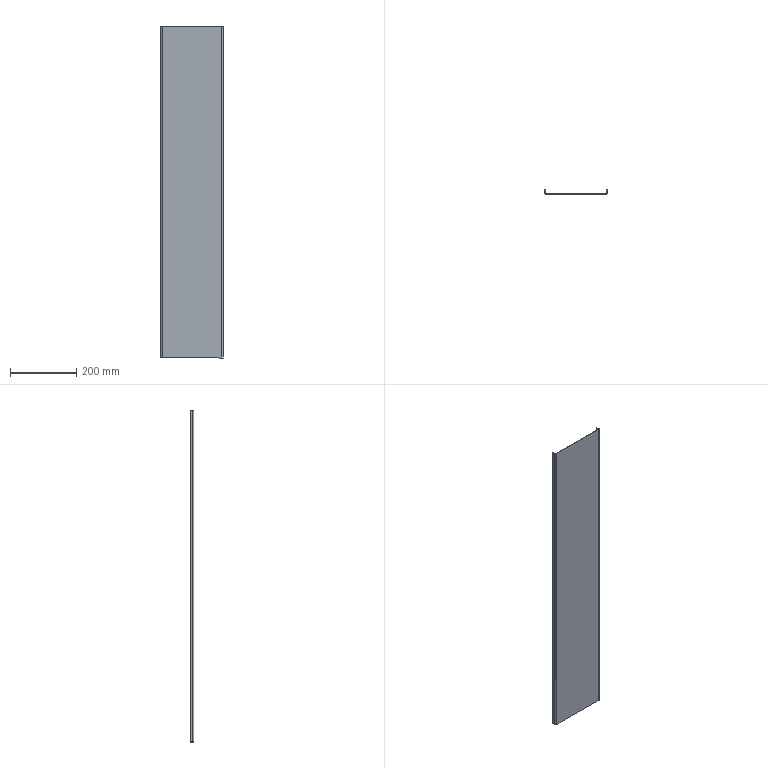Part | STEP file | HXGR200008-05-16 | 1 solid | 22 faces | box 187 x 12 x 1000 mm | volume 408850 mm3 | plane 18 | cylinder 4 | commonest cylinder face diameters 4 x2 8 x2
STEP:
#1=CARTESIAN_POINT('',(-91.5,2.,-1000.));
#2=VERTEX_POINT('',#1);
#3=CARTESIAN_POINT('',(-93.5,2.,-1000.));
#4=VERTEX_POINT('',#3);
#5=CARTESIAN_POINT('',(-91.5,2.,-1000.));
#6=DIRECTION('',(-1.,0.,0.));
#7=VECTOR('',#6,1000.);
#8=LINE('',#5,#7);
#9=EDGE_CURVE('',#2,#4,#8,.T.);
#10=ORIENTED_EDGE('',*,*,#9,.F.);
#11=CARTESIAN_POINT('',(-89.5,0.,-1000.));
#12=VERTEX_POINT('',#11);
#13=CARTESIAN_POINT('',(-89.5,2.,-1000.));
#14=DIRECTION('',(0.,0.,1.));
#15=DIRECTION('',(-1.,0.,0.));
#16=AXIS2_PLACEMENT_3D('',#13,#14,#15);
#17=CIRCLE('',#16,2.);
#18=EDGE_CURVE('',#2,#12,#17,.T.);
#19=ORIENTED_EDGE('',*,*,#18,.T.);
#20=CARTESIAN_POINT('',(-89.5,-2.,-1000.));
#21=VERTEX_POINT('',#20);
#22=CARTESIAN_POINT('',(-89.5,-2.,-1000.));
#23=DIRECTION('',(0.,1.,0.));
#24=VECTOR('',#23,1000.);
#25=LINE('',#22,#24);
#26=EDGE_CURVE('',#21,#12,#25,.T.);
#27=ORIENTED_EDGE('',*,*,#26,.F.);
#28=CARTESIAN_POINT('',(-89.5,2.,-1000.));
#29=DIRECTION('',(0.,0.,1.));
#30=DIRECTION('',(1.,0.,0.));
#31=AXIS2_PLACEMENT_3D('',#28,#29,#30);
#32=CIRCLE('',#31,4.);
#33=EDGE_CURVE('',#4,#21,#32,.T.);
#34=ORIENTED_EDGE('',*,*,#33,.F.);
#35=EDGE_LOOP('',(#10,#19,#27,#34));
#36=FACE_OUTER_BOUND('',#35,.T.);
#37=CARTESIAN_POINT('',(-91.5,2.,-1000.));
#38=DIRECTION('',(0.,0.,-1.));
#39=DIRECTION('',(-1.,0.,0.));
#40=AXIS2_PLACEMENT_3D('',#37,#38,#39);
#41=PLANE('',#40);
#42=ADVANCED_FACE('',(#36),#41,.T.);
#43=CARTESIAN_POINT('',(-91.5,10.,-1000.));
#44=VERTEX_POINT('',#43);
#45=CARTESIAN_POINT('',(-91.5,0.,-1000.));
#46=DIRECTION('',(0.,-1.,0.));
#47=VECTOR('',#46,1000.);
#48=LINE('',#45,#47);
#49=EDGE_CURVE('',#44,#2,#48,.T.);
#50=ORIENTED_EDGE('',*,*,#49,.T.);
#51=ORIENTED_EDGE('',*,*,#9,.T.);
#52=CARTESIAN_POINT('',(-93.5,10.,-1000.));
#53=VERTEX_POINT('',#52);
#54=CARTESIAN_POINT('',(-93.5,0.,-1000.));
#55=DIRECTION('',(0.,-1.,0.));
#56=VECTOR('',#55,1000.);
#57=LINE('',#54,#56);
#58=EDGE_CURVE('',#53,#4,#57,.T.);
#59=ORIENTED_EDGE('',*,*,#58,.F.);
#60=CARTESIAN_POINT('',(-93.5,10.,-1000.));
#61=DIRECTION('',(1.,0.,0.));
#62=VECTOR('',#61,1000.);
#63=LINE('',#60,#62);
#64=EDGE_CURVE('',#53,#44,#63,.T.);
#65=ORIENTED_EDGE('',*,*,#64,.T.);
#66=EDGE_LOOP('',(#50,#51,#59,#65));
#67=FACE_OUTER_BOUND('',#66,.T.);
#68=CARTESIAN_POINT('',(-89.5,-2.,-1000.));
#69=DIRECTION('',(0.,0.,-1.));
#70=DIRECTION('',(-1.,0.,0.));
#71=AXIS2_PLACEMENT_3D('',#68,#69,#70);
#72=PLANE('',#71);
#73=ADVANCED_FACE('',(#67),#72,.T.);
#74=CARTESIAN_POINT('',(-89.5,0.,0.));
#75=VERTEX_POINT('',#74);
#76=CARTESIAN_POINT('',(-89.5,-2.,0.));
#77=VERTEX_POINT('',#76);
#78=CARTESIAN_POINT('',(-89.5,0.,0.));
#79=DIRECTION('',(0.,-1.,0.));
#80=VECTOR('',#79,1000.);
#81=LINE('',#78,#80);
#82=EDGE_CURVE('',#75,#77,#81,.T.);
#83=ORIENTED_EDGE('',*,*,#82,.F.);
#84=CARTESIAN_POINT('',(-91.5,2.,0.));
#85=VERTEX_POINT('',#84);
#86=CARTESIAN_POINT('',(-89.5,2.,0.));
#87=DIRECTION('',(0.,0.,1.));
#88=DIRECTION('',(-1.,0.,0.));
#89=AXIS2_PLACEMENT_3D('',#86,#87,#88);
#90=CIRCLE('',#89,2.);
#91=EDGE_CURVE('',#85,#75,#90,.T.);
#92=ORIENTED_EDGE('',*,*,#91,.F.);
#93=CARTESIAN_POINT('',(-93.5,2.,0.));
#94=VERTEX_POINT('',#93);
#95=CARTESIAN_POINT('',(-93.5,2.,0.));
#96=DIRECTION('',(1.,0.,0.));
#97=VECTOR('',#96,1000.);
#98=LINE('',#95,#97);
#99=EDGE_CURVE('',#94,#85,#98,.T.);
#100=ORIENTED_EDGE('',*,*,#99,.F.);
#101=CARTESIAN_POINT('',(-89.5,2.,0.));
#102=DIRECTION('',(0.,0.,1.));
#103=DIRECTION('',(1.,0.,0.));
#104=AXIS2_PLACEMENT_3D('',#101,#102,#103);
#105=CIRCLE('',#104,4.);
#106=EDGE_CURVE('',#94,#77,#105,.T.);
#107=ORIENTED_EDGE('',*,*,#106,.T.);
#108=EDGE_LOOP('',(#83,#92,#100,#107));
#109=FACE_OUTER_BOUND('',#108,.T.);
#110=CARTESIAN_POINT('',(-89.5,0.,0.));
#111=DIRECTION('',(0.,0.,1.));
#112=DIRECTION('',(1.,0.,0.));
#113=AXIS2_PLACEMENT_3D('',#110,#111,#112);
#114=PLANE('',#113);
#115=ADVANCED_FACE('',(#109),#114,.T.);
#116=CARTESIAN_POINT('',(89.5,0.,0.));
#117=VERTEX_POINT('',#116);
#118=CARTESIAN_POINT('',(-91.5,0.,0.));
#119=DIRECTION('',(1.,0.,0.));
#120=VECTOR('',#119,1000.);
#121=LINE('',#118,#120);
#122=EDGE_CURVE('',#75,#117,#121,.T.);
#123=ORIENTED_EDGE('',*,*,#122,.F.);
#124=ORIENTED_EDGE('',*,*,#82,.T.);
#125=CARTESIAN_POINT('',(89.5,-2.,0.));
#126=VERTEX_POINT('',#125);
#127=CARTESIAN_POINT('',(-91.5,-2.,0.));
#128=DIRECTION('',(1.,0.,0.));
#129=VECTOR('',#128,1000.);
#130=LINE('',#127,#129);
#131=EDGE_CURVE('',#77,#126,#130,.T.);
#132=ORIENTED_EDGE('',*,*,#131,.T.);
#133=CARTESIAN_POINT('',(89.5,-2.,0.));
#134=DIRECTION('',(0.,1.,0.));
#135=VECTOR('',#134,1000.);
#136=LINE('',#133,#135);
#137=EDGE_CURVE('',#126,#117,#136,.T.);
#138=ORIENTED_EDGE('',*,*,#137,.T.);
#139=EDGE_LOOP('',(#123,#124,#132,#138));
#140=FACE_OUTER_BOUND('',#139,.T.);
#141=CARTESIAN_POINT('',(-93.5,2.,0.));
#142=DIRECTION('',(0.,0.,1.));
#143=DIRECTION('',(1.,0.,0.));
#144=AXIS2_PLACEMENT_3D('',#141,#142,#143);
#145=PLANE('',#144);
#146=ADVANCED_FACE('',(#140),#145,.T.);
#147=CARTESIAN_POINT('',(89.5,0.,-1000.));
#148=VERTEX_POINT('',#147);
#149=CARTESIAN_POINT('',(89.5,-2.,-1000.));
#150=VERTEX_POINT('',#149);
#151=CARTESIAN_POINT('',(89.5,0.,-1000.));
#152=DIRECTION('',(0.,-1.,0.));
#153=VECTOR('',#152,1000.);
#154=LINE('',#151,#153);
#155=EDGE_CURVE('',#148,#150,#154,.T.);
#156=ORIENTED_EDGE('',*,*,#155,.F.);
#157=CARTESIAN_POINT('',(91.5,2.,-1000.));
#158=VERTEX_POINT('',#157);
#159=CARTESIAN_POINT('',(89.5,2.,-1000.));
#160=DIRECTION('',(0.,0.,1.));
#161=DIRECTION('',(-1.,0.,0.));
#162=AXIS2_PLACEMENT_3D('',#159,#160,#161);
#163=CIRCLE('',#162,2.);
#164=EDGE_CURVE('',#148,#158,#163,.T.);
#165=ORIENTED_EDGE('',*,*,#164,.T.);
#166=CARTESIAN_POINT('',(93.5,2.,-1000.));
#167=VERTEX_POINT('',#166);
#168=CARTESIAN_POINT('',(93.5,2.,-1000.));
#169=DIRECTION('',(-1.,0.,0.));
#170=VECTOR('',#169,1000.);
#171=LINE('',#168,#170);
#172=EDGE_CURVE('',#167,#158,#171,.T.);
#173=ORIENTED_EDGE('',*,*,#172,.F.);
#174=CARTESIAN_POINT('',(89.5,2.,-1000.));
#175=DIRECTION('',(0.,0.,1.));
#176=DIRECTION('',(1.,0.,0.));
#177=AXIS2_PLACEMENT_3D('',#174,#175,#176);
#178=CIRCLE('',#177,4.);
#179=EDGE_CURVE('',#150,#167,#178,.T.);
#180=ORIENTED_EDGE('',*,*,#179,.F.);
#181=EDGE_LOOP('',(#156,#165,#173,#180));
#182=FACE_OUTER_BOUND('',#181,.T.);
#183=CARTESIAN_POINT('',(89.5,0.,-1000.));
#184=DIRECTION('',(0.,0.,-1.));
#185=DIRECTION('',(-1.,0.,0.));
#186=AXIS2_PLACEMENT_3D('',#183,#184,#185);
#187=PLANE('',#186);
#188=ADVANCED_FACE('',(#182),#187,.T.);
#189=CARTESIAN_POINT('',(-91.5,0.,-1000.));
#190=DIRECTION('',(1.,0.,0.));
#191=VECTOR('',#190,1000.);
#192=LINE('',#189,#191);
#193=EDGE_CURVE('',#12,#148,#192,.T.);
#194=ORIENTED_EDGE('',*,*,#193,.T.);
#195=ORIENTED_EDGE('',*,*,#155,.T.);
#196=CARTESIAN_POINT('',(-91.5,-2.,-1000.));
#197=DIRECTION('',(1.,0.,0.));
#198=VECTOR('',#197,1000.);
#199=LINE('',#196,#198);
#200=EDGE_CURVE('',#21,#150,#199,.T.);
#201=ORIENTED_EDGE('',*,*,#200,.F.);
#202=ORIENTED_EDGE('',*,*,#26,.T.);
#203=EDGE_LOOP('',(#194,#195,#201,#202));
#204=FACE_OUTER_BOUND('',#203,.T.);
#205=CARTESIAN_POINT('',(93.5,2.,-1000.));
#206=DIRECTION('',(0.,0.,-1.));
#207=DIRECTION('',(-1.,0.,0.));
#208=AXIS2_PLACEMENT_3D('',#205,#206,#207);
#209=PLANE('',#208);
#210=ADVANCED_FACE('',(#204),#209,.T.);
#211=CARTESIAN_POINT('',(91.5,2.,0.));
#212=VERTEX_POINT('',#211);
#213=CARTESIAN_POINT('',(93.5,2.,0.));
#214=VERTEX_POINT('',#213);
#215=CARTESIAN_POINT('',(91.5,2.,0.));
#216=DIRECTION('',(1.,0.,0.));
#217=VECTOR('',#216,1000.);
#218=LINE('',#215,#217);
#219=EDGE_CURVE('',#212,#214,#218,.T.);
#220=ORIENTED_EDGE('',*,*,#219,.F.);
#221=CARTESIAN_POINT('',(89.5,2.,0.));
#222=DIRECTION('',(0.,0.,1.));
#223=DIRECTION('',(-1.,0.,0.));
#224=AXIS2_PLACEMENT_3D('',#221,#222,#223);
#225=CIRCLE('',#224,2.);
#226=EDGE_CURVE('',#117,#212,#225,.T.);
#227=ORIENTED_EDGE('',*,*,#226,.F.);
#228=ORIENTED_EDGE('',*,*,#137,.F.);
#229=CARTESIAN_POINT('',(89.5,2.,0.));
#230=DIRECTION('',(0.,0.,1.));
#231=DIRECTION('',(1.,0.,0.));
#232=AXIS2_PLACEMENT_3D('',#229,#230,#231);
#233=CIRCLE('',#232,4.);
#234=EDGE_CURVE('',#126,#214,#233,.T.);
#235=ORIENTED_EDGE('',*,*,#234,.T.);
#236=EDGE_LOOP('',(#220,#227,#228,#235));
#237=FACE_OUTER_BOUND('',#236,.T.);
#238=CARTESIAN_POINT('',(91.5,2.,0.));
#239=DIRECTION('',(0.,0.,1.));
#240=DIRECTION('',(1.,0.,0.));
#241=AXIS2_PLACEMENT_3D('',#238,#239,#240);
#242=PLANE('',#241);
#243=ADVANCED_FACE('',(#237),#242,.T.);
#244=CARTESIAN_POINT('',(91.5,10.,0.));
#245=VERTEX_POINT('',#244);
#246=CARTESIAN_POINT('',(91.5,0.,0.));
#247=DIRECTION('',(0.,1.,0.));
#248=VECTOR('',#247,1000.);
#249=LINE('',#246,#248);
#250=EDGE_CURVE('',#212,#245,#249,.T.);
#251=ORIENTED_EDGE('',*,*,#250,.F.);
#252=ORIENTED_EDGE('',*,*,#219,.T.);
#253=CARTESIAN_POINT('',(93.5,10.,0.));
#254=VERTEX_POINT('',#253);
#255=CARTESIAN_POINT('',(93.5,0.,0.));
#256=DIRECTION('',(0.,1.,0.));
#257=VECTOR('',#256,1000.);
#258=LINE('',#255,#257);
#259=EDGE_CURVE('',#214,#254,#258,.T.);
#260=ORIENTED_EDGE('',*,*,#259,.T.);
#261=CARTESIAN_POINT('',(91.5,10.,0.));
#262=DIRECTION('',(1.,0.,0.));
#263=VECTOR('',#262,1000.);
#264=LINE('',#261,#263);
#265=EDGE_CURVE('',#245,#254,#264,.T.);
#266=ORIENTED_EDGE('',*,*,#265,.F.);
#267=EDGE_LOOP('',(#251,#252,#260,#266));
#268=FACE_OUTER_BOUND('',#267,.T.);
#269=CARTESIAN_POINT('',(89.5,-2.,0.));
#270=DIRECTION('',(0.,0.,1.));
#271=DIRECTION('',(1.,0.,0.));
#272=AXIS2_PLACEMENT_3D('',#269,#270,#271);
#273=PLANE('',#272);
#274=ADVANCED_FACE('',(#268),#273,.T.);
#275=ORIENTED_EDGE('',*,*,#259,.F.);
#276=CARTESIAN_POINT('',(93.5,2.,-1000.));
#277=DIRECTION('',(0.,0.,1.));
#278=VECTOR('',#277,1000.);
#279=LINE('',#276,#278);
#280=EDGE_CURVE('',#167,#214,#279,.T.);
#281=ORIENTED_EDGE('',*,*,#280,.F.);
#282=CARTESIAN_POINT('',(93.5,10.,-1000.));
#283=VERTEX_POINT('',#282);
#284=CARTESIAN_POINT('',(93.5,0.,-1000.));
#285=DIRECTION('',(0.,1.,0.));
#286=VECTOR('',#285,1000.);
#287=LINE('',#284,#286);
#288=EDGE_CURVE('',#167,#283,#287,.T.);
#289=ORIENTED_EDGE('',*,*,#288,.T.);
#290=CARTESIAN_POINT('',(93.5,10.,-1000.));
#291=DIRECTION('',(0.,0.,1.));
#292=VECTOR('',#291,1000.);
#293=LINE('',#290,#292);
#294=EDGE_CURVE('',#283,#254,#293,.T.);
#295=ORIENTED_EDGE('',*,*,#294,.T.);
#296=EDGE_LOOP('',(#275,#281,#289,#295));
#297=FACE_OUTER_BOUND('',#296,.T.);
#298=CARTESIAN_POINT('',(93.5,0.,-1000.));
#299=DIRECTION('',(1.,0.,0.));
#300=DIRECTION('',(0.,0.,-1.));
#301=AXIS2_PLACEMENT_3D('',#298,#299,#300);
#302=PLANE('',#301);
#303=ADVANCED_FACE('',(#297),#302,.T.);
#304=ORIENTED_EDGE('',*,*,#234,.F.);
#305=CARTESIAN_POINT('',(89.5,-2.,-1000.));
#306=DIRECTION('',(0.,0.,1.));
#307=VECTOR('',#306,1000.);
#308=LINE('',#305,#307);
#309=EDGE_CURVE('',#150,#126,#308,.T.);
#310=ORIENTED_EDGE('',*,*,#309,.F.);
#311=ORIENTED_EDGE('',*,*,#179,.T.);
#312=ORIENTED_EDGE('',*,*,#280,.T.);
#313=EDGE_LOOP('',(#304,#310,#311,#312));
#314=FACE_OUTER_BOUND('',#313,.T.);
#315=CARTESIAN_POINT('',(89.5,2.,-1000.));
#316=DIRECTION('',(0.,0.,1.));
#317=DIRECTION('',(1.,0.,0.));
#318=AXIS2_PLACEMENT_3D('',#315,#316,#317);
#319=CYLINDRICAL_SURFACE('',#318,4.);
#320=ADVANCED_FACE('',(#314),#319,.T.);
#321=ORIENTED_EDGE('',*,*,#131,.F.);
#322=CARTESIAN_POINT('',(-89.5,-2.,-1000.));
#323=DIRECTION('',(0.,0.,1.));
#324=VECTOR('',#323,1000.);
#325=LINE('',#322,#324);
#326=EDGE_CURVE('',#21,#77,#325,.T.);
#327=ORIENTED_EDGE('',*,*,#326,.F.);
#328=ORIENTED_EDGE('',*,*,#200,.T.);
#329=ORIENTED_EDGE('',*,*,#309,.T.);
#330=EDGE_LOOP('',(#321,#327,#328,#329));
#331=FACE_OUTER_BOUND('',#330,.T.);
#332=CARTESIAN_POINT('',(-91.5,-2.,-1000.));
#333=DIRECTION('',(0.,-1.,0.));
#334=DIRECTION('',(1.,0.,0.));
#335=AXIS2_PLACEMENT_3D('',#332,#333,#334);
#336=PLANE('',#335);
#337=ADVANCED_FACE('',(#331),#336,.T.);
#338=ORIENTED_EDGE('',*,*,#106,.F.);
#339=CARTESIAN_POINT('',(-93.5,2.,-1000.));
#340=DIRECTION('',(0.,0.,1.));
#341=VECTOR('',#340,1000.);
#342=LINE('',#339,#341);
#343=EDGE_CURVE('',#4,#94,#342,.T.);
#344=ORIENTED_EDGE('',*,*,#343,.F.);
#345=ORIENTED_EDGE('',*,*,#33,.T.);
#346=ORIENTED_EDGE('',*,*,#326,.T.);
#347=EDGE_LOOP('',(#338,#344,#345,#346));
#348=FACE_OUTER_BOUND('',#347,.T.);
#349=CARTESIAN_POINT('',(-89.5,2.,-1000.));
#350=DIRECTION('',(0.,0.,1.));
#351=DIRECTION('',(1.,0.,0.));
#352=AXIS2_PLACEMENT_3D('',#349,#350,#351);
#353=CYLINDRICAL_SURFACE('',#352,4.);
#354=ADVANCED_FACE('',(#348),#353,.T.);
#355=CARTESIAN_POINT('',(-93.5,10.,0.));
#356=VERTEX_POINT('',#355);
#357=CARTESIAN_POINT('',(-93.5,0.,0.));
#358=DIRECTION('',(0.,-1.,0.));
#359=VECTOR('',#358,1000.);
#360=LINE('',#357,#359);
#361=EDGE_CURVE('',#356,#94,#360,.T.);
#362=ORIENTED_EDGE('',*,*,#361,.F.);
#363=CARTESIAN_POINT('',(-93.5,10.,-1000.));
#364=DIRECTION('',(0.,0.,1.));
#365=VECTOR('',#364,1000.);
#366=LINE('',#363,#365);
#367=EDGE_CURVE('',#53,#356,#366,.T.);
#368=ORIENTED_EDGE('',*,*,#367,.F.);
#369=ORIENTED_EDGE('',*,*,#58,.T.);
#370=ORIENTED_EDGE('',*,*,#343,.T.);
#371=EDGE_LOOP('',(#362,#368,#369,#370));
#372=FACE_OUTER_BOUND('',#371,.T.);
#373=CARTESIAN_POINT('',(-93.5,0.,-1000.));
#374=DIRECTION('',(-1.,0.,0.));
#375=DIRECTION('',(0.,0.,1.));
#376=AXIS2_PLACEMENT_3D('',#373,#374,#375);
#377=PLANE('',#376);
#378=ADVANCED_FACE('',(#372),#377,.T.);
#379=CARTESIAN_POINT('',(-91.5,10.,0.));
#380=VERTEX_POINT('',#379);
#381=CARTESIAN_POINT('',(-93.5,10.,0.));
#382=DIRECTION('',(1.,0.,0.));
#383=VECTOR('',#382,1000.);
#384=LINE('',#381,#383);
#385=EDGE_CURVE('',#356,#380,#384,.T.);
#386=ORIENTED_EDGE('',*,*,#385,.T.);
#387=CARTESIAN_POINT('',(-91.5,10.,-1000.));
#388=DIRECTION('',(0.,0.,1.));
#389=VECTOR('',#388,1000.);
#390=LINE('',#387,#389);
#391=EDGE_CURVE('',#44,#380,#390,.T.);
#392=ORIENTED_EDGE('',*,*,#391,.F.);
#393=ORIENTED_EDGE('',*,*,#64,.F.);
#394=ORIENTED_EDGE('',*,*,#367,.T.);
#395=EDGE_LOOP('',(#386,#392,#393,#394));
#396=FACE_OUTER_BOUND('',#395,.T.);
#397=CARTESIAN_POINT('',(-93.5,10.,-1000.));
#398=DIRECTION('',(0.,-1.,0.));
#399=DIRECTION('',(0.,0.,-1.));
#400=AXIS2_PLACEMENT_3D('',#397,#398,#399);
#401=PLANE('',#400);
#402=ADVANCED_FACE('',(#396),#401,.F.);
#403=CARTESIAN_POINT('',(-91.5,0.,0.));
#404=DIRECTION('',(0.,-1.,0.));
#405=VECTOR('',#404,1000.);
#406=LINE('',#403,#405);
#407=EDGE_CURVE('',#380,#85,#406,.T.);
#408=ORIENTED_EDGE('',*,*,#407,.T.);
#409=CARTESIAN_POINT('',(-91.5,2.,-1000.));
#410=DIRECTION('',(0.,0.,1.));
#411=VECTOR('',#410,1000.);
#412=LINE('',#409,#411);
#413=EDGE_CURVE('',#2,#85,#412,.T.);
#414=ORIENTED_EDGE('',*,*,#413,.F.);
#415=ORIENTED_EDGE('',*,*,#49,.F.);
#416=ORIENTED_EDGE('',*,*,#391,.T.);
#417=EDGE_LOOP('',(#408,#414,#415,#416));
#418=FACE_OUTER_BOUND('',#417,.T.);
#419=CARTESIAN_POINT('',(-91.5,0.,-1000.));
#420=DIRECTION('',(-1.,0.,0.));
#421=DIRECTION('',(0.,0.,1.));
#422=AXIS2_PLACEMENT_3D('',#419,#420,#421);
#423=PLANE('',#422);
#424=ADVANCED_FACE('',(#418),#423,.F.);
#425=ORIENTED_EDGE('',*,*,#91,.T.);
#426=CARTESIAN_POINT('',(-89.5,0.,-1000.));
#427=DIRECTION('',(0.,0.,1.));
#428=VECTOR('',#427,1000.);
#429=LINE('',#426,#428);
#430=EDGE_CURVE('',#12,#75,#429,.T.);
#431=ORIENTED_EDGE('',*,*,#430,.F.);
#432=ORIENTED_EDGE('',*,*,#18,.F.);
#433=ORIENTED_EDGE('',*,*,#413,.T.);
#434=EDGE_LOOP('',(#425,#431,#432,#433));
#435=FACE_OUTER_BOUND('',#434,.T.);
#436=CARTESIAN_POINT('',(-89.5,2.,-1000.));
#437=DIRECTION('',(0.,0.,1.));
#438=DIRECTION('',(1.,0.,0.));
#439=AXIS2_PLACEMENT_3D('',#436,#437,#438);
#440=CYLINDRICAL_SURFACE('',#439,2.);
#441=ADVANCED_FACE('',(#435),#440,.F.);
#442=ORIENTED_EDGE('',*,*,#122,.T.);
#443=CARTESIAN_POINT('',(89.5,0.,-1000.));
#444=DIRECTION('',(0.,0.,1.));
#445=VECTOR('',#444,1000.);
#446=LINE('',#443,#445);
#447=EDGE_CURVE('',#148,#117,#446,.T.);
#448=ORIENTED_EDGE('',*,*,#447,.F.);
#449=ORIENTED_EDGE('',*,*,#193,.F.);
#450=ORIENTED_EDGE('',*,*,#430,.T.);
#451=EDGE_LOOP('',(#442,#448,#449,#450));
#452=FACE_OUTER_BOUND('',#451,.T.);
#453=CARTESIAN_POINT('',(-91.5,0.,-1000.));
#454=DIRECTION('',(0.,-1.,0.));
#455=DIRECTION('',(1.,0.,0.));
#456=AXIS2_PLACEMENT_3D('',#453,#454,#455);
#457=PLANE('',#456);
#458=ADVANCED_FACE('',(#452),#457,.F.);
#459=ORIENTED_EDGE('',*,*,#226,.T.);
#460=CARTESIAN_POINT('',(91.5,2.,-1000.));
#461=DIRECTION('',(0.,0.,1.));
#462=VECTOR('',#461,1000.);
#463=LINE('',#460,#462);
#464=EDGE_CURVE('',#158,#212,#463,.T.);
#465=ORIENTED_EDGE('',*,*,#464,.F.);
#466=ORIENTED_EDGE('',*,*,#164,.F.);
#467=ORIENTED_EDGE('',*,*,#447,.T.);
#468=EDGE_LOOP('',(#459,#465,#466,#467));
#469=FACE_OUTER_BOUND('',#468,.T.);
#470=CARTESIAN_POINT('',(89.5,2.,-1000.));
#471=DIRECTION('',(0.,0.,1.));
#472=DIRECTION('',(1.,0.,0.));
#473=AXIS2_PLACEMENT_3D('',#470,#471,#472);
#474=CYLINDRICAL_SURFACE('',#473,2.);
#475=ADVANCED_FACE('',(#469),#474,.F.);
#476=ORIENTED_EDGE('',*,*,#250,.T.);
#477=CARTESIAN_POINT('',(91.5,10.,-1000.));
#478=VERTEX_POINT('',#477);
#479=CARTESIAN_POINT('',(91.5,10.,-1000.));
#480=DIRECTION('',(0.,0.,1.));
#481=VECTOR('',#480,1000.);
#482=LINE('',#479,#481);
#483=EDGE_CURVE('',#478,#245,#482,.T.);
#484=ORIENTED_EDGE('',*,*,#483,.F.);
#485=CARTESIAN_POINT('',(91.5,0.,-1000.));
#486=DIRECTION('',(0.,1.,0.));
#487=VECTOR('',#486,1000.);
#488=LINE('',#485,#487);
#489=EDGE_CURVE('',#158,#478,#488,.T.);
#490=ORIENTED_EDGE('',*,*,#489,.F.);
#491=ORIENTED_EDGE('',*,*,#464,.T.);
#492=EDGE_LOOP('',(#476,#484,#490,#491));
#493=FACE_OUTER_BOUND('',#492,.T.);
#494=CARTESIAN_POINT('',(91.5,0.,-1000.));
#495=DIRECTION('',(1.,0.,0.));
#496=DIRECTION('',(0.,0.,-1.));
#497=AXIS2_PLACEMENT_3D('',#494,#495,#496);
#498=PLANE('',#497);
#499=ADVANCED_FACE('',(#493),#498,.F.);
#500=ORIENTED_EDGE('',*,*,#265,.T.);
#501=ORIENTED_EDGE('',*,*,#294,.F.);
#502=CARTESIAN_POINT('',(91.5,10.,-1000.));
#503=DIRECTION('',(1.,0.,0.));
#504=VECTOR('',#503,1000.);
#505=LINE('',#502,#504);
#506=EDGE_CURVE('',#478,#283,#505,.T.);
#507=ORIENTED_EDGE('',*,*,#506,.F.);
#508=ORIENTED_EDGE('',*,*,#483,.T.);
#509=EDGE_LOOP('',(#500,#501,#507,#508));
#510=FACE_OUTER_BOUND('',#509,.T.);
#511=CARTESIAN_POINT('',(91.5,10.,-1000.));
#512=DIRECTION('',(0.,-1.,0.));
#513=DIRECTION('',(0.,0.,-1.));
#514=AXIS2_PLACEMENT_3D('',#511,#512,#513);
#515=PLANE('',#514);
#516=ADVANCED_FACE('',(#510),#515,.F.);
#517=ORIENTED_EDGE('',*,*,#288,.F.);
#518=ORIENTED_EDGE('',*,*,#172,.T.);
#519=ORIENTED_EDGE('',*,*,#489,.T.);
#520=ORIENTED_EDGE('',*,*,#506,.T.);
#521=EDGE_LOOP('',(#517,#518,#519,#520));
#522=FACE_OUTER_BOUND('',#521,.T.);
#523=CARTESIAN_POINT('',(89.5,2.,-1000.));
#524=DIRECTION('',(0.,0.,-1.));
#525=DIRECTION('',(-1.,0.,0.));
#526=AXIS2_PLACEMENT_3D('',#523,#524,#525);
#527=PLANE('',#526);
#528=ADVANCED_FACE('',(#522),#527,.T.);
#529=ORIENTED_EDGE('',*,*,#361,.T.);
#530=ORIENTED_EDGE('',*,*,#99,.T.);
#531=ORIENTED_EDGE('',*,*,#407,.F.);
#532=ORIENTED_EDGE('',*,*,#385,.F.);
#533=EDGE_LOOP('',(#529,#530,#531,#532));
#534=FACE_OUTER_BOUND('',#533,.T.);
#535=CARTESIAN_POINT('',(89.5,2.,0.));
#536=DIRECTION('',(0.,0.,-1.));
#537=DIRECTION('',(-1.,0.,0.));
#538=AXIS2_PLACEMENT_3D('',#535,#536,#537);
#539=PLANE('',#538);
#540=ADVANCED_FACE('',(#534),#539,.F.);
#541=CLOSED_SHELL('',(#42,#73,#115,#146,#188,#210,#243,#274,#303,#320,#337,#354,#378,#402,#424,#441,#458,#475,#499,#516,#528,#540));
#542=MANIFOLD_SOLID_BREP('',#541);
#543=CARTESIAN_POINT('',(0.,0.,0.));
#544=DIRECTION('',(0.,0.,1.));
#545=DIRECTION('',(1.,0.,0.));
#546=AXIS2_PLACEMENT_3D('',#543,#544,#545);
#547=(LENGTH_UNIT()NAMED_UNIT(*)SI_UNIT(.MILLI.,.METRE.));
#548=UNCERTAINTY_MEASURE_WITH_UNIT(LENGTH_MEASURE(0.00001),#547,'','');
#549=(NAMED_UNIT(*)PLANE_ANGLE_UNIT()SI_UNIT($,.RADIAN.));
#550=(NAMED_UNIT(*)SI_UNIT($,.STERADIAN.)SOLID_ANGLE_UNIT());
#551=(GEOMETRIC_REPRESENTATION_CONTEXT(3)GLOBAL_UNCERTAINTY_ASSIGNED_CONTEXT((#548))GLOBAL_UNIT_ASSIGNED_CONTEXT((#547,#549,#550))REPRESENTATION_CONTEXT('',''));
#552=ADVANCED_BREP_SHAPE_REPRESENTATION('',(#542,#546),#551);